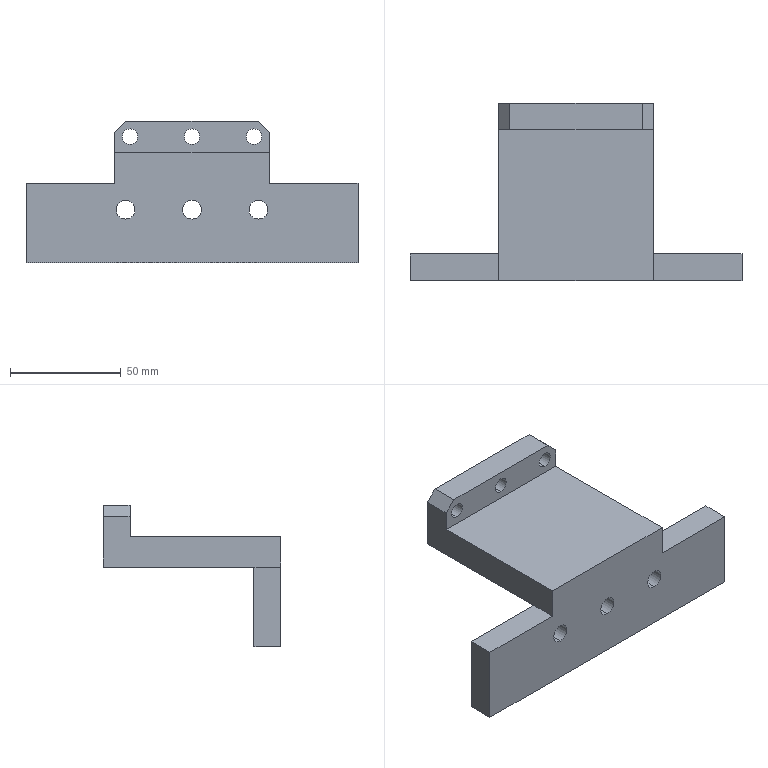NC program | NX | posted with a generic post | part box 150 x 80 x 64 mm
Whole program, first 2936 of 3152 lines:
N10 G17 G21 G94 G90
(FLOOR_WALL_COPY , TOOL : D63)
N12 T01 M6
N14 G54
N16 G17 G0 G90 X111.5 Y-41.997 B0. C0. S6500 M3
N18 G43 Z30. H1
N20 Z3.
N22 G94 G1 Z0. F1250.
N24 X108.5
N26 X-108.5
N28 Y-32.188
N30 Y-12.599
N32 X108.5
N34 Y16.8
N36 X-108.5
N38 X-111.5
N40 Z3.
N42 G0 Z30.
N44 M5
(FLOOR_WALL_2 , TOOL : D10)
N46 T10 M6
N48 G54
N50 G17 G0 G90 X1.443 Y-46.5 B0. C0. S9500 M3
N52 G43 Z30. H10
N54 Z1.001
N56 G94 G1 Z-0.499 F1000.
N58 X0.866 Y-45.5
N60 G3 X0. Y-45. R1.
N62 G1 X-40. F2500.
N64 Y22.9
N66 X40.
N68 Y-45.
N70 X0.
N72 Y-39.
N74 X-34.
N76 Y16.9
N78 X34.
N80 Y-39.
N82 X0.
N84 Y-33.
N86 X-28.
N88 Y10.9
N90 X28.
N92 Y-33.
N94 X0.
N96 Y-27.
N98 X-22.
N100 Y4.9
N102 X22.
N104 Y-27.
N106 X0.
N108 Y-21.
N110 X-16.
N112 Y-1.1
N114 X16.
N116 Y-21.
N118 X0.
N120 Y-15.
N122 X-10.
N124 Y-7.1
N126 X10.
N128 Y-15.
N130 X0.
N132 G3 X-0.866 Y-15.5 R1.
N134 G1 Z1.001
N136 G0 Z30.
N138 X1.443 Y-46.5
N140 Z0.503
N142 G1 Z-0.997 F1000.
N144 X0.866 Y-45.5
N146 G3 X0. Y-45. R1.
N148 G1 X-40. F2500.
N150 Y22.9
N152 X40.
N154 Y-45.
N156 X0.
N158 Y-39.
N160 X-34.
N162 Y16.9
N164 X34.
N166 Y-39.
N168 X0.
N170 Y-33.
N172 X-28.
N174 Y10.9
N176 X28.
N178 Y-33.
N180 X0.
N182 Y-27.
N184 X-22.
N186 Y4.9
N188 X22.
N190 Y-27.
N192 X0.
N194 Y-21.
N196 X-16.
N198 Y-1.1
N200 X16.
N202 Y-21.
N204 X0.
N206 Y-15.
N208 X-10.
N210 Y-7.1
N212 X10.
N214 Y-15.
N216 X0.
N218 G3 X-0.866 Y-15.5 R1.
N220 G1 Z0.503
N222 G0 Z30.
N224 X1.443 Y-46.5
N226 Z0.004
N228 G1 Z-1.496 F1000.
N230 X0.866 Y-45.5
N232 G3 X0. Y-45. R1.
N234 G1 X-40. F2500.
N236 Y22.9
N238 X40.
N240 Y-45.
N242 X0.
N244 Y-39.
N246 X-34.
N248 Y16.9
N250 X34.
N252 Y-39.
N254 X0.
N256 Y-33.
N258 X-28.
N260 Y10.9
N262 X28.
N264 Y-33.
N266 X0.
N268 Y-27.
N270 X-22.
N272 Y4.9
N274 X22.
N276 Y-27.
N278 X0.
N280 Y-21.
N282 X-16.
N284 Y-1.1
N286 X16.
N288 Y-21.
N290 X0.
N292 Y-15.
N294 X-10.
N296 Y-7.1
N298 X10.
N300 Y-15.
N302 X0.
N304 G3 X-0.866 Y-15.5 R1.
N306 G1 Z0.004
N308 G0 Z30.
N310 X1.443 Y-46.5
N312 Z-0.494
N314 G1 Z-1.994 F1000.
N316 X0.866 Y-45.5
N318 G3 X0. Y-45. R1.
N320 G1 X-40. F2500.
N322 Y22.9
N324 X40.
N326 Y-45.
N328 X0.
N330 Y-39.
N332 X-34.
N334 Y16.9
N336 X34.
N338 Y-39.
N340 X0.
N342 Y-33.
N344 X-28.
N346 Y10.9
N348 X28.
N350 Y-33.
N352 X0.
N354 Y-27.
N356 X-22.
N358 Y4.9
N360 X22.
N362 Y-27.
N364 X0.
N366 Y-21.
N368 X-16.
N370 Y-1.1
N372 X16.
N374 Y-21.
N376 X0.
N378 Y-15.
N380 X-10.
N382 Y-7.1
N384 X10.
N386 Y-15.
N388 X0.
N390 G3 X-0.866 Y-15.5 R1.
N392 G1 Z-0.494
N394 G0 Z30.
N396 X1.443 Y-46.5
N398 Z-0.993
N400 G1 Z-2.493 F1000.
N402 X0.866 Y-45.5
N404 G3 X0. Y-45. R1.
N406 G1 X-40. F2500.
N408 Y22.9
N410 X40.
N412 Y-45.
N414 X0.
N416 Y-39.
N418 X-34.
N420 Y16.9
N422 X34.
N424 Y-39.
N426 X0.
N428 Y-33.
N430 X-28.
N432 Y10.9
N434 X28.
N436 Y-33.
N438 X0.
N440 Y-27.
N442 X-22.
N444 Y4.9
N446 X22.
N448 Y-27.
N450 X0.
N452 Y-21.
N454 X-16.
N456 Y-1.1
N458 X16.
N460 Y-21.
N462 X0.
N464 Y-15.
N466 X-10.
N468 Y-7.1
N470 X10.
N472 Y-15.
N474 X0.
N476 G3 X-0.866 Y-15.5 R1.
N478 G1 Z-0.993
N480 G0 Z30.
N482 X1.443 Y-46.5
N484 Z-1.492
N486 G1 Z-2.992 F1000.
N488 X0.866 Y-45.5
N490 G3 X0. Y-45. R1.
N492 G1 X-40. F2500.
N494 Y22.9
N496 X40.
N498 Y-45.
N500 X0.
N502 Y-39.
N504 X-34.
N506 Y16.9
N508 X34.
N510 Y-39.
N512 X0.
N514 Y-33.
N516 X-28.
N518 Y10.9
N520 X28.
N522 Y-33.
N524 X0.
N526 Y-27.
N528 X-22.
N530 Y4.9
N532 X22.
N534 Y-27.
N536 X0.
N538 Y-21.
N540 X-16.
N542 Y-1.1
N544 X16.
N546 Y-21.
N548 X0.
N550 Y-15.
N552 X-10.
N554 Y-7.1
N556 X10.
N558 Y-15.
N560 X0.
N562 G3 X-0.866 Y-15.5 R1.
N564 G1 Z-1.492
N566 G0 Z30.
N568 X1.443 Y-46.5
N570 Z-1.99
N572 G1 Z-3.49 F1000.
N574 X0.866 Y-45.5
N576 G3 X0. Y-45. R1.
N578 G1 X-40. F2500.
N580 Y22.9
N582 X40.
N584 Y-45.
N586 X0.
N588 Y-39.
N590 X-34.
N592 Y16.9
N594 X34.
N596 Y-39.
N598 X0.
N600 Y-33.
N602 X-28.
N604 Y10.9
N606 X28.
N608 Y-33.
N610 X0.
N612 Y-27.
N614 X-22.
N616 Y4.9
N618 X22.
N620 Y-27.
N622 X0.
N624 Y-21.
N626 X-16.
N628 Y-1.1
N630 X16.
N632 Y-21.
N634 X0.
N636 Y-15.
N638 X-10.
N640 Y-7.1
N642 X10.
N644 Y-15.
N646 X0.
N648 G3 X-0.866 Y-15.5 R1.
N650 G1 Z-1.99
N652 G0 Z30.
N654 X1.443 Y-46.5
N656 Z-2.489
N658 G1 Z-3.989 F1000.
N660 X0.866 Y-45.5
N662 G3 X0. Y-45. R1.
N664 G1 X-40. F2500.
N666 Y22.9
N668 X40.
N670 Y-45.
N672 X0.
N674 Y-39.
N676 X-34.
N678 Y16.9
N680 X34.
N682 Y-39.
N684 X0.
N686 Y-33.
N688 X-28.
N690 Y10.9
N692 X28.
N694 Y-33.
N696 X0.
N698 Y-27.
N700 X-22.
N702 Y4.9
N704 X22.
N706 Y-27.
N708 X0.
N710 Y-21.
N712 X-16.
N714 Y-1.1
N716 X16.
N718 Y-21.
N720 X0.
N722 Y-15.
N724 X-10.
N726 Y-7.1
N728 X10.
N730 Y-15.
N732 X0.
N734 G3 X-0.866 Y-15.5 R1.
N736 G1 Z-2.489
N738 G0 Z30.
N740 X1.443 Y-46.5
N742 Z-2.988
N744 G1 Z-4.488 F1000.
N746 X0.866 Y-45.5
N748 G3 X0. Y-45. R1.
N750 G1 X-40. F2500.
N752 Y22.9
N754 X40.
N756 Y-45.
N758 X0.
N760 Y-39.
N762 X-34.
N764 Y16.9
N766 X34.
N768 Y-39.
N770 X0.
N772 Y-33.
N774 X-28.
N776 Y10.9
N778 X28.
N780 Y-33.
N782 X0.
N784 Y-27.
N786 X-22.
N788 Y4.9
N790 X22.
N792 Y-27.
N794 X0.
N796 Y-21.
N798 X-16.
N800 Y-1.1
N802 X16.
N804 Y-21.
N806 X0.
N808 Y-15.
N810 X-10.
N812 Y-7.1
N814 X10.
N816 Y-15.
N818 X0.
N820 G3 X-0.866 Y-15.5 R1.
N822 G1 Z-2.988
N824 G0 Z30.
N826 X1.443 Y-46.5
N828 Z-3.486
N830 G1 Z-4.986 F1000.
N832 X0.866 Y-45.5
N834 G3 X0. Y-45. R1.
N836 G1 X-40. F2500.
N838 Y22.9
N840 X40.
N842 Y-45.
N844 X0.
N846 Y-39.
N848 X-34.
N850 Y16.9
N852 X34.
N854 Y-39.
N856 X0.
N858 Y-33.
N860 X-28.
N862 Y10.9
N864 X28.
N866 Y-33.
N868 X0.
N870 Y-27.
N872 X-22.
N874 Y4.9
N876 X22.
N878 Y-27.
N880 X0.
N882 Y-21.
N884 X-16.
N886 Y-1.1
N888 X16.
N890 Y-21.
N892 X0.
N894 Y-15.
N896 X-10.
N898 Y-7.1
N900 X10.
N902 Y-15.
N904 X0.
N906 G3 X-0.866 Y-15.5 R1.
N908 G1 Z-3.486
N910 G0 Z30.
N912 X1.443 Y-46.5
N914 Z-3.985
N916 G1 Z-5.485 F1000.
N918 X0.866 Y-45.5
N920 G3 X0. Y-45. R1.
N922 G1 X-40. F2500.
N924 Y22.9
N926 X40.
N928 Y-45.
N930 X0.
N932 Y-39.
N934 X-34.
N936 Y16.9
N938 X34.
N940 Y-39.
N942 X0.
N944 Y-33.
N946 X-28.
N948 Y10.9
N950 X28.
N952 Y-33.
N954 X0.
N956 Y-27.
N958 X-22.
N960 Y4.9
N962 X22.
N964 Y-27.
N966 X0.
N968 Y-21.
N970 X-16.
N972 Y-1.1
N974 X16.
N976 Y-21.
N978 X0.
N980 Y-15.
N982 X-10.
N984 Y-7.1
N986 X10.
N988 Y-15.
N990 X0.
N992 G3 X-0.866 Y-15.5 R1.
N994 G1 Z-3.985
N996 G0 Z30.
N998 X1.443 Y-46.5
N1000 Z-4.483
N1002 G1 Z-5.983 F1000.
N1004 X0.866 Y-45.5
N1006 G3 X0. Y-45. R1.
N1008 G1 X-40. F2500.
N1010 Y22.9
N1012 X40.
N1014 Y-45.
N1016 X0.
N1018 Y-39.
N1020 X-34.
N1022 Y16.9
N1024 X34.
N1026 Y-39.
N1028 X0.
N1030 Y-33.
N1032 X-28.
N1034 Y10.9
N1036 X28.
N1038 Y-33.
N1040 X0.
N1042 Y-27.
N1044 X-22.
N1046 Y4.9
N1048 X22.
N1050 Y-27.
N1052 X0.
N1054 Y-21.
N1056 X-16.
N1058 Y-1.1
N1060 X16.
N1062 Y-21.
N1064 X0.
N1066 Y-15.
N1068 X-10.
N1070 Y-7.1
N1072 X10.
N1074 Y-15.
N1076 X0.
N1078 G3 X-0.866 Y-15.5 R1.
N1080 G1 Z-4.483
N1082 G0 Z30.
N1084 X1.443 Y-46.5
N1086 Z-4.982
N1088 G1 Z-6.482 F1000.
N1090 X0.866 Y-45.5
N1092 G3 X0. Y-45. R1.
N1094 G1 X-40. F2500.
N1096 Y22.9
N1098 X40.
N1100 Y-45.
N1102 X0.
N1104 Y-39.
N1106 X-34.
N1108 Y16.9
N1110 X34.
N1112 Y-39.
N1114 X0.
N1116 Y-33.
N1118 X-28.
N1120 Y10.9
N1122 X28.
N1124 Y-33.
N1126 X0.
N1128 Y-27.
N1130 X-22.
N1132 Y4.9
N1134 X22.
N1136 Y-27.
N1138 X0.
N1140 Y-21.
N1142 X-16.
N1144 Y-1.1
N1146 X16.
N1148 Y-21.
N1150 X0.
N1152 Y-15.
N1154 X-10.
N1156 Y-7.1
N1158 X10.
N1160 Y-15.
N1162 X0.
N1164 G3 X-0.866 Y-15.5 R1.
N1166 G1 Z-4.982
N1168 G0 Z30.
N1170 X1.443 Y-46.5
N1172 Z-5.481
N1174 G1 Z-6.981 F1000.
N1176 X0.866 Y-45.5
N1178 G3 X0. Y-45. R1.
N1180 G1 X-40. F2500.
N1182 Y22.9
N1184 X40.
N1186 Y-45.
N1188 X0.
N1190 Y-39.
N1192 X-34.
N1194 Y16.9
N1196 X34.
N1198 Y-39.
N1200 X0.
N1202 Y-33.
N1204 X-28.
N1206 Y10.9
N1208 X28.
N1210 Y-33.
N1212 X0.
N1214 Y-27.
N1216 X-22.
N1218 Y4.9
N1220 X22.
N1222 Y-27.
N1224 X0.
N1226 Y-21.
N1228 X-16.
N1230 Y-1.1
N1232 X16.
N1234 Y-21.
N1236 X0.
N1238 Y-15.
N1240 X-10.
N1242 Y-7.1
N1244 X10.
N1246 Y-15.
N1248 X0.
N1250 G3 X-0.866 Y-15.5 R1.
N1252 G1 Z-5.481
N1254 G0 Z30.
N1256 X1.443 Y-46.5
N1258 Z-5.979
N1260 G1 Z-7.479 F1000.
N1262 X0.866 Y-45.5
N1264 G3 X0. Y-45. R1.
N1266 G1 X-40. F2500.
N1268 Y22.9
N1270 X40.
N1272 Y-45.
N1274 X0.
N1276 Y-39.
N1278 X-34.
N1280 Y16.9
N1282 X34.
N1284 Y-39.
N1286 X0.
N1288 Y-33.
N1290 X-28.
N1292 Y10.9
N1294 X28.
N1296 Y-33.
N1298 X0.
N1300 Y-27.
N1302 X-22.
N1304 Y4.9
N1306 X22.
N1308 Y-27.
N1310 X0.
N1312 Y-21.
N1314 X-16.
N1316 Y-1.1
N1318 X16.
N1320 Y-21.
N1322 X0.
N1324 Y-15.
N1326 X-10.
N1328 Y-7.1
N1330 X10.
N1332 Y-15.
N1334 X0.
N1336 G3 X-0.866 Y-15.5 R1.
N1338 G1 Z-5.979
N1340 G0 Z30.
N1342 X1.443 Y-46.5
N1344 Z-6.478
N1346 G1 Z-7.978 F1000.
N1348 X0.866 Y-45.5
N1350 G3 X0. Y-45. R1.
N1352 G1 X-40. F2500.
N1354 Y22.9
N1356 X40.
N1358 Y-45.
N1360 X0.
N1362 Y-39.
N1364 X-34.
N1366 Y16.9
N1368 X34.
N1370 Y-39.
N1372 X0.
N1374 Y-33.
N1376 X-28.
N1378 Y10.9
N1380 X28.
N1382 Y-33.
N1384 X0.
N1386 Y-27.
N1388 X-22.
N1390 Y4.9
N1392 X22.
N1394 Y-27.
N1396 X0.
N1398 Y-21.
N1400 X-16.
N1402 Y-1.1
N1404 X16.
N1406 Y-21.
N1408 X0.
N1410 Y-15.
N1412 X-10.
N1414 Y-7.1
N1416 X10.
N1418 Y-15.
N1420 X0.
N1422 G3 X-0.866 Y-15.5 R1.
N1424 G1 Z-6.478
N1426 G0 Z30.
N1428 X1.443 Y-46.5
N1430 Z-6.976
N1432 G1 Z-8.476 F1000.
N1434 X0.866 Y-45.5
N1436 G3 X0. Y-45. R1.
N1438 G1 X-40. F2500.
N1440 Y22.9
N1442 X40.
N1444 Y-45.
N1446 X0.
N1448 Y-39.
N1450 X-34.
N1452 Y16.9
N1454 X34.
N1456 Y-39.
N1458 X0.
N1460 Y-33.
N1462 X-28.
N1464 Y10.9
N1466 X28.
N1468 Y-33.
N1470 X0.
N1472 Y-27.
N1474 X-22.
N1476 Y4.9
N1478 X22.
N1480 Y-27.
N1482 X0.
N1484 Y-21.
N1486 X-16.
N1488 Y-1.1
N1490 X16.
N1492 Y-21.
N1494 X0.
N1496 Y-15.
N1498 X-10.
N1500 Y-7.1
N1502 X10.
N1504 Y-15.
N1506 X0.
N1508 G3 X-0.866 Y-15.5 R1.
N1510 G1 Z-6.976
N1512 G0 Z30.
N1514 X1.443 Y-46.5
N1516 Z-7.475
N1518 G1 Z-8.975 F1000.
N1520 X0.866 Y-45.5
N1522 G3 X0. Y-45. R1.
N1524 G1 X-40. F2500.
N1526 Y22.9
N1528 X40.
N1530 Y-45.
N1532 X0.
N1534 Y-39.
N1536 X-34.
N1538 Y16.9
N1540 X34.
N1542 Y-39.
N1544 X0.
N1546 Y-33.
N1548 X-28.
N1550 Y10.9
N1552 X28.
N1554 Y-33.
N1556 X0.
N1558 Y-27.
N1560 X-22.
N1562 Y4.9
N1564 X22.
N1566 Y-27.
N1568 X0.
N1570 Y-21.
N1572 X-16.
N1574 Y-1.1
N1576 X16.
N1578 Y-21.
N1580 X0.
N1582 Y-15.
N1584 X-10.
N1586 Y-7.1
N1588 X10.
N1590 Y-15.
N1592 X0.
N1594 G3 X-0.866 Y-15.5 R1.
N1596 G1 Z-7.475
N1598 G0 Z30.
N1600 X1.443 Y-46.5
N1602 Z-7.974
N1604 G1 Z-9.474 F1000.
N1606 X0.866 Y-45.5
N1608 G3 X0. Y-45. R1.
N1610 G1 X-40. F2500.
N1612 Y22.9
N1614 X40.
N1616 Y-45.
N1618 X0.
N1620 Y-39.
N1622 X-34.
N1624 Y16.9
N1626 X34.
N1628 Y-39.
N1630 X0.
N1632 Y-33.
N1634 X-28.
N1636 Y10.9
N1638 X28.
N1640 Y-33.
N1642 X0.
N1644 Y-27.
N1646 X-22.
N1648 Y4.9
N1650 X22.
N1652 Y-27.
N1654 X0.
N1656 Y-21.
N1658 X-16.
N1660 Y-1.1
N1662 X16.
N1664 Y-21.
N1666 X0.
N1668 Y-15.
N1670 X-10.
N1672 Y-7.1
N1674 X10.
N1676 Y-15.
N1678 X0.
N1680 G3 X-0.866 Y-15.5 R1.
N1682 G1 Z-7.974
N1684 G0 Z30.
N1686 X1.443 Y-46.5
N1688 Z-8.472
N1690 G1 Z-9.972 F1000.
N1692 X0.866 Y-45.5
N1694 G3 X0. Y-45. R1.
N1696 G1 X-40. F2500.
N1698 Y22.9
N1700 X40.
N1702 Y-45.
N1704 X0.
N1706 Y-39.
N1708 X-34.
N1710 Y16.9
N1712 X34.
N1714 Y-39.
N1716 X0.
N1718 Y-33.
N1720 X-28.
N1722 Y10.9
N1724 X28.
N1726 Y-33.
N1728 X0.
N1730 Y-27.
N1732 X-22.
N1734 Y4.9
N1736 X22.
N1738 Y-27.
N1740 X0.
N1742 Y-21.
N1744 X-16.
N1746 Y-1.1
N1748 X16.
N1750 Y-21.
N1752 X0.
N1754 Y-15.
N1756 X-10.
N1758 Y-7.1
N1760 X10.
N1762 Y-15.
N1764 X0.
N1766 G3 X-0.866 Y-15.5 R1.
N1768 G1 Z-8.472
N1770 G0 Z30.
N1772 X1.443 Y-46.5
N1774 Z-8.971
N1776 G1 Z-10.471 F1000.
N1778 X0.866 Y-45.5
N1780 G3 X0. Y-45. R1.
N1782 G1 X-40. F2500.
N1784 Y22.9
N1786 X40.
N1788 Y-45.
N1790 X0.
N1792 Y-39.
N1794 X-34.
N1796 Y16.9
N1798 X34.
N1800 Y-39.
N1802 X0.
N1804 Y-33.
N1806 X-28.
N1808 Y10.9
N1810 X28.
N1812 Y-33.
N1814 X0.
N1816 Y-27.
N1818 X-22.
N1820 Y4.9
N1822 X22.
N1824 Y-27.
N1826 X0.
N1828 Y-21.
N1830 X-16.
N1832 Y-1.1
N1834 X16.
N1836 Y-21.
N1838 X0.
N1840 Y-15.
N1842 X-10.
N1844 Y-7.1
N1846 X10.
N1848 Y-15.
N1850 X0.
N1852 G3 X-0.866 Y-15.5 R1.
N1854 G1 Z-8.971
N1856 G0 Z30.
N1858 X1.443 Y-46.5
N1860 Z-9.469
N1862 G1 Z-10.969 F1000.
N1864 X0.866 Y-45.5
N1866 G3 X0. Y-45. R1.
N1868 G1 X-40. F2500.
N1870 Y22.9
N1872 X40.
N1874 Y-45.
N1876 X0.
N1878 Y-39.
N1880 X-34.
N1882 Y16.9
N1884 X34.
N1886 Y-39.
N1888 X0.
N1890 Y-33.
N1892 X-28.
N1894 Y10.9
N1896 X28.
N1898 Y-33.
N1900 X0.
N1902 Y-27.
N1904 X-22.
N1906 Y4.9
N1908 X22.
N1910 Y-27.
N1912 X0.
N1914 Y-21.
N1916 X-16.
N1918 Y-1.1
N1920 X16.
N1922 Y-21.
N1924 X0.
N1926 Y-15.
N1928 X-10.
N1930 Y-7.1
N1932 X10.
N1934 Y-15.
N1936 X0.
N1938 G3 X-0.866 Y-15.5 R1.
N1940 G1 Z-9.469
N1942 G0 Z30.
N1944 X1.443 Y-46.5
N1946 Z-9.968
N1948 G1 Z-11.468 F1000.
N1950 X0.866 Y-45.5
N1952 G3 X0. Y-45. R1.
N1954 G1 X-40. F2500.
N1956 Y22.9
N1958 X40.
N1960 Y-45.
N1962 X0.
N1964 Y-39.
N1966 X-34.
N1968 Y16.9
N1970 X34.
N1972 Y-39.
N1974 X0.
N1976 Y-33.
N1978 X-28.
N1980 Y10.9
N1982 X28.
N1984 Y-33.
N1986 X0.
N1988 Y-27.
N1990 X-22.
N1992 Y4.9
N1994 X22.
N1996 Y-27.
N1998 X0.
N2000 Y-21.
N2002 X-16.
N2004 Y-1.1
N2006 X16.
N2008 Y-21.
N2010 X0.
N2012 Y-15.
N2014 X-10.
N2016 Y-7.1
N2018 X10.
N2020 Y-15.
N2022 X0.
N2024 G3 X-0.866 Y-15.5 R1.
N2026 G1 Z-9.968
N2028 G0 Z30.
N2030 X1.443 Y-46.5
N2032 Z-10.467
N2034 G1 Z-11.967 F1000.
N2036 X0.866 Y-45.5
N2038 G3 X0. Y-45. R1.
N2040 G1 X-40. F2500.
N2042 Y22.9
N2044 X40.
N2046 Y-45.
N2048 X0.
N2050 Y-39.
N2052 X-34.
N2054 Y16.9
N2056 X34.
N2058 Y-39.
N2060 X0.
N2062 Y-33.
N2064 X-28.
N2066 Y10.9
N2068 X28.
N2070 Y-33.
N2072 X0.
N2074 Y-27.
N2076 X-22.
N2078 Y4.9
N2080 X22.
N2082 Y-27.
N2084 X0.
N2086 Y-21.
N2088 X-16.
N2090 Y-1.1
N2092 X16.
N2094 Y-21.
N2096 X0.
N2098 Y-15.
N2100 X-10.
N2102 Y-7.1
N2104 X10.
N2106 Y-15.
N2108 X0.
N2110 G3 X-0.866 Y-15.5 R1.
N2112 G1 Z-10.467
N2114 G0 Z30.
N2116 X1.443 Y-46.5
N2118 Z-10.965
N2120 G1 Z-12.465 F1000.
N2122 X0.866 Y-45.5
N2124 G3 X0. Y-45. R1.
N2126 G1 X-40. F2500.
N2128 Y22.9
N2130 X40.
N2132 Y-45.
N2134 X0.
N2136 Y-39.
N2138 X-34.
N2140 Y16.9
N2142 X34.
N2144 Y-39.
N2146 X0.
N2148 Y-33.
N2150 X-28.
N2152 Y10.9
N2154 X28.
N2156 Y-33.
N2158 X0.
N2160 Y-27.
N2162 X-22.
N2164 Y4.9
N2166 X22.
N2168 Y-27.
N2170 X0.
N2172 Y-21.
N2174 X-16.
N2176 Y-1.1
N2178 X16.
N2180 Y-21.
N2182 X0.
N2184 Y-15.
N2186 X-10.
N2188 Y-7.1
N2190 X10.
N2192 Y-15.
N2194 X0.
N2196 G3 X-0.866 Y-15.5 R1.
N2198 G1 Z-10.965
N2200 G0 Z30.
N2202 X1.443 Y-46.5
N2204 Z-11.464
N2206 G1 Z-12.964 F1000.
N2208 X0.866 Y-45.5
N2210 G3 X0. Y-45. R1.
N2212 G1 X-40. F2500.
N2214 Y22.9
N2216 X40.
N2218 Y-45.
N2220 X0.
N2222 Y-39.
N2224 X-34.
N2226 Y16.9
N2228 X34.
N2230 Y-39.
N2232 X0.
N2234 Y-33.
N2236 X-28.
N2238 Y10.9
N2240 X28.
N2242 Y-33.
N2244 X0.
N2246 Y-27.
N2248 X-22.
N2250 Y4.9
N2252 X22.
N2254 Y-27.
N2256 X0.
N2258 Y-21.
N2260 X-16.
N2262 Y-1.1
N2264 X16.
N2266 Y-21.
N2268 X0.
N2270 Y-15.
N2272 X-10.
N2274 Y-7.1
N2276 X10.
N2278 Y-15.
N2280 X0.
N2282 G3 X-0.866 Y-15.5 R1.
N2284 G1 Z-11.464
N2286 G0 Z30.
N2288 X1.443 Y-46.5
N2290 Z-11.963
N2292 G1 Z-13.463 F1000.
N2294 X0.866 Y-45.5
N2296 G3 X0. Y-45. R1.
N2298 G1 X-40. F2500.
N2300 Y22.9
N2302 X40.
N2304 Y-45.
N2306 X0.
N2308 Y-39.
N2310 X-34.
N2312 Y16.9
N2314 X34.
N2316 Y-39.
N2318 X0.
N2320 Y-33.
N2322 X-28.
N2324 Y10.9
N2326 X28.
N2328 Y-33.
N2330 X0.
N2332 Y-27.
N2334 X-22.
N2336 Y4.9
N2338 X22.
N2340 Y-27.
N2342 X0.
N2344 Y-21.
N2346 X-16.
N2348 Y-1.1
N2350 X16.
N2352 Y-21.
N2354 X0.
N2356 Y-15.
N2358 X-10.
N2360 Y-7.1
N2362 X10.
N2364 Y-15.
N2366 X0.
N2368 G3 X-0.866 Y-15.5 R1.
N2370 G1 Z-11.963
N2372 G0 Z30.
N2374 X1.443 Y-46.5
N2376 Z-12.461
N2378 G1 Z-13.961 F1000.
N2380 X0.866 Y-45.5
N2382 G3 X0. Y-45. R1.
N2384 G1 X-40. F2500.
N2386 Y22.9
N2388 X40.
N2390 Y-45.
N2392 X0.
N2394 Y-39.
N2396 X-34.
N2398 Y16.9
N2400 X34.
N2402 Y-39.
N2404 X0.
N2406 Y-33.
N2408 X-28.
N2410 Y10.9
N2412 X28.
N2414 Y-33.
N2416 X0.
N2418 Y-27.
N2420 X-22.
N2422 Y4.9
N2424 X22.
N2426 Y-27.
N2428 X0.
N2430 Y-21.
N2432 X-16.
N2434 Y-1.1
N2436 X16.
N2438 Y-21.
N2440 X0.
N2442 Y-15.
N2444 X-10.
N2446 Y-7.1
N2448 X10.
N2450 Y-15.
N2452 X0.
N2454 G3 X-0.866 Y-15.5 R1.
N2456 G1 Z-12.461
N2458 G0 Z30.
N2460 X1.443 Y-46.5
N2462 Z-12.96
N2464 G1 Z-14.46 F1000.
N2466 X0.866 Y-45.5
N2468 G3 X0. Y-45. R1.
N2470 G1 X-40. F2500.
N2472 Y22.9
N2474 X40.
N2476 Y-45.
N2478 X0.
N2480 Y-39.
N2482 X-34.
N2484 Y16.9
N2486 X34.
N2488 Y-39.
N2490 X0.
N2492 Y-33.
N2494 X-28.
N2496 Y10.9
N2498 X28.
N2500 Y-33.
N2502 X0.
N2504 Y-27.
N2506 X-22.
N2508 Y4.9
N2510 X22.
N2512 Y-27.
N2514 X0.
N2516 Y-21.
N2518 X-16.
N2520 Y-1.1
N2522 X16.
N2524 Y-21.
N2526 X0.
N2528 Y-15.
N2530 X-10.
N2532 Y-7.1
N2534 X10.
N2536 Y-15.
N2538 X0.
N2540 G3 X-0.866 Y-15.5 R1.
N2542 G1 Z-12.96
N2544 G0 Z30.
N2546 X1.443 Y-46.5
N2548 Z-13.458
N2550 G1 Z-14.958 F1000.
N2552 X0.866 Y-45.5
N2554 G3 X0. Y-45. R1.
N2556 G1 X-40. F2500.
N2558 Y22.9
N2560 X40.
N2562 Y-45.
N2564 X0.
N2566 Y-39.
N2568 X-34.
N2570 Y16.9
N2572 X34.
N2574 Y-39.
N2576 X0.
N2578 Y-33.
N2580 X-28.
N2582 Y10.9
N2584 X28.
N2586 Y-33.
N2588 X0.
N2590 Y-27.
N2592 X-22.
N2594 Y4.9
N2596 X22.
N2598 Y-27.
N2600 X0.
N2602 Y-21.
N2604 X-16.
N2606 Y-1.1
N2608 X16.
N2610 Y-21.
N2612 X0.
N2614 Y-15.
N2616 X-10.
N2618 Y-7.1
N2620 X10.
N2622 Y-15.
N2624 X0.
N2626 G3 X-0.866 Y-15.5 R1.
N2628 G1 Z-13.458
N2630 G0 Z30.
N2632 X1.443 Y-46.5
N2634 Z-13.957
N2636 G1 Z-15.457 F1000.
N2638 X0.866 Y-45.5
N2640 G3 X0. Y-45. R1.
N2642 G1 X-40. F2500.
N2644 Y22.9
N2646 X40.
N2648 Y-45.
N2650 X0.
N2652 Y-39.
N2654 X-34.
N2656 Y16.9
N2658 X34.
N2660 Y-39.
N2662 X0.
N2664 Y-33.
N2666 X-28.
N2668 Y10.9
N2670 X28.
N2672 Y-33.
N2674 X0.
N2676 Y-27.
N2678 X-22.
N2680 Y4.9
N2682 X22.
N2684 Y-27.
N2686 X0.
N2688 Y-21.
N2690 X-16.
N2692 Y-1.1
N2694 X16.
N2696 Y-21.
N2698 X0.
N2700 Y-15.
N2702 X-10.
N2704 Y-7.1
N2706 X10.
N2708 Y-15.
N2710 X0.
N2712 G3 X-0.866 Y-15.5 R1.
N2714 G1 Z-13.957
N2716 G0 Z30.
N2718 X1.443 Y-46.5
N2720 Z-14.456
N2722 G1 Z-15.956 F1000.
N2724 X0.866 Y-45.5
N2726 G3 X0. Y-45. R1.
N2728 G1 X-40. F2500.
N2730 Y22.9
N2732 X40.
N2734 Y-45.
N2736 X0.
N2738 Y-39.
N2740 X-34.
N2742 Y16.9
N2744 X34.
N2746 Y-39.
N2748 X0.
N2750 Y-33.
N2752 X-28.
N2754 Y10.9
N2756 X28.
N2758 Y-33.
N2760 X0.
N2762 Y-27.
N2764 X-22.
N2766 Y4.9
N2768 X22.
N2770 Y-27.
N2772 X0.
N2774 Y-21.
N2776 X-16.
N2778 Y-1.1
N2780 X16.
N2782 Y-21.
N2784 X0.
N2786 Y-15.
N2788 X-10.
N2790 Y-7.1
N2792 X10.
N2794 Y-15.
N2796 X0.
N2798 G3 X-0.866 Y-15.5 R1.
N2800 G1 Z-14.456
N2802 G0 Z30.
N2804 X1.443 Y-46.5
N2806 Z-14.954
N2808 G1 Z-16.454 F1000.
N2810 X0.866 Y-45.5
N2812 G3 X0. Y-45. R1.
N2814 G1 X-40. F2500.
N2816 Y22.9
N2818 X40.
N2820 Y-45.
N2822 X0.
N2824 Y-39.
N2826 X-34.
N2828 Y16.9
N2830 X34.
N2832 Y-39.
N2834 X0.
N2836 Y-33.
N2838 X-28.
N2840 Y10.9
N2842 X28.
N2844 Y-33.
N2846 X0.
N2848 Y-27.
N2850 X-22.
N2852 Y4.9
N2854 X22.
N2856 Y-27.
N2858 X0.
N2860 Y-21.
N2862 X-16.
N2864 Y-1.1
N2866 X16.
N2868 Y-21.
N2870 X0.
N2872 Y-15.
N2874 X-10.
N2876 Y-7.1
N2878 X10.
N2880 Y-15.
N2882 X0.
N2884 G3 X-0.866 Y-15.5 R1.
N2886 G1 Z-14.954
N2888 G0 Z30.
N2890 X1.443 Y-46.5
N2892 Z-15.453
N2894 G1 Z-16.953 F1000.
N2896 X0.866 Y-45.5
N2898 G3 X0. Y-45. R1.
N2900 G1 X-40. F2500.
N2902 Y22.9
N2904 X40.
N2906 Y-45.
N2908 X0.
N2910 Y-39.
N2912 X-34.
N2914 Y16.9
N2916 X34.
N2918 Y-39.
N2920 X0.
N2922 Y-33.
N2924 X-28.
N2926 Y10.9
N2928 X28.
N2930 Y-33.
N2932 X0.
N2934 Y-27.
N2936 X-22.
N2938 Y4.9
N2940 X22.
N2942 Y-27.
N2944 X0.
N2946 Y-21.
N2948 X-16.
N2950 Y-1.1
N2952 X16.
N2954 Y-21.
N2956 X0.
N2958 Y-15.
N2960 X-10.
N2962 Y-7.1
N2964 X10.
N2966 Y-15.
N2968 X0.
N2970 G3 X-0.866 Y-15.5 R1.
N2972 G1 Z-15.453
N2974 G0 Z30.
N2976 X1.443 Y-46.5
N2978 Z-15.951
N2980 G1 Z-17.451 F1000.
N2982 X0.866 Y-45.5
N2984 G3 X0. Y-45. R1.
N2986 G1 X-40. F2500.
N2988 Y22.9
N2990 X40.
N2992 Y-45.
N2994 X0.
N2996 Y-39.
N2998 X-34.
N3000 Y16.9
N3002 X34.
N3004 Y-39.
N3006 X0.
N3008 Y-33.
N3010 X-28.
N3012 Y10.9
N3014 X28.
N3016 Y-33.
N3018 X0.
N3020 Y-27.
N3022 X-22.
N3024 Y4.9
N3026 X22.
N3028 Y-27.
N3030 X0.
N3032 Y-21.
N3034 X-16.
N3036 Y-1.1
N3038 X16.
N3040 Y-21.
N3042 X0.
N3044 Y-15.
N3046 X-10.
N3048 Y-7.1
N3050 X10.
N3052 Y-15.
N3054 X0.
N3056 G3 X-0.866 Y-15.5 R1.
N3058 G1 Z-15.951
N3060 G0 Z30.
N3062 X1.443 Y-46.5
N3064 Z-16.45
N3066 G1 Z-17.95 F1000.
N3068 X0.866 Y-45.5
N3070 G3 X0. Y-45. R1.
N3072 G1 X-40. F2500.
N3074 Y22.9
N3076 X40.
N3078 Y-45.
N3080 X0.
N3082 Y-39.
N3084 X-34.
N3086 Y16.9
N3088 X34.
N3090 Y-39.
N3092 X0.
N3094 Y-33.
N3096 X-28.
N3098 Y10.9
N3100 X28.
N3102 Y-33.
N3104 X0.
N3106 Y-27.
N3108 X-22.
N3110 Y4.9
N3112 X22.
N3114 Y-27.
N3116 X0.
N3118 Y-21.
N3120 X-16.
N3122 Y-1.1
N3124 X16.
N3126 Y-21.
N3128 X0.
N3130 Y-15.
N3132 X-10.
N3134 Y-7.1
N3136 X10.
N3138 Y-15.
N3140 X0.
N3142 G3 X-0.866 Y-15.5 R1.
N3144 G1 Z-16.45
N3146 G0 Z30.
N3148 X1.443 Y-46.5
N3150 Z-16.949
N3152 G1 Z-18.449 F1000.
N3154 X0.866 Y-45.5
N3156 G3 X0. Y-45. R1.
N3158 G1 X-40. F2500.
N3160 Y22.9
N3162 X40.
N3164 Y-45.
N3166 X0.
N3168 Y-39.
N3170 X-34.
N3172 Y16.9
N3174 X34.
N3176 Y-39.
N3178 X0.
N3180 Y-33.
N3182 X-28.
N3184 Y10.9
N3186 X28.
N3188 Y-33.
N3190 X0.
N3192 Y-27.
N3194 X-22.
N3196 Y4.9
N3198 X22.
N3200 Y-27.
N3202 X0.
N3204 Y-21.
N3206 X-16.
N3208 Y-1.1
N3210 X16.
N3212 Y-21.
N3214 X0.
N3216 Y-15.
N3218 X-10.
N3220 Y-7.1
N3222 X10.
N3224 Y-15.
N3226 X0.
N3228 G3 X-0.866 Y-15.5 R1.
N3230 G1 Z-16.949
N3232 G0 Z30.
N3234 X1.443 Y-46.5
N3236 Z-17.447
N3238 G1 Z-18.947 F1000.
N3240 X0.866 Y-45.5
N3242 G3 X0. Y-45. R1.
N3244 G1 X-40. F2500.
N3246 Y22.9
N3248 X40.
N3250 Y-45.
N3252 X0.
N3254 Y-39.
N3256 X-34.
N3258 Y16.9
N3260 X34.
N3262 Y-39.
N3264 X0.
N3266 Y-33.
N3268 X-28.
N3270 Y10.9
N3272 X28.
N3274 Y-33.
N3276 X0.
N3278 Y-27.
N3280 X-22.
N3282 Y4.9
N3284 X22.
N3286 Y-27.
N3288 X0.
N3290 Y-21.
N3292 X-16.
N3294 Y-1.1
N3296 X16.
N3298 Y-21.
N3300 X0.
N3302 Y-15.
N3304 X-10.
N3306 Y-7.1
N3308 X10.
N3310 Y-15.
N3312 X0.
N3314 G3 X-0.866 Y-15.5 R1.
N3316 G1 Z-17.447
N3318 G0 Z30.
N3320 X1.443 Y-46.5
N3322 Z-17.946
N3324 G1 Z-19.446 F1000.
N3326 X0.866 Y-45.5
N3328 G3 X0. Y-45. R1.
N3330 G1 X-40. F2500.
N3332 Y22.9
N3334 X40.
N3336 Y-45.
N3338 X0.
N3340 Y-39.
N3342 X-34.
N3344 Y16.9
N3346 X34.
N3348 Y-39.
N3350 X0.
N3352 Y-33.
N3354 X-28.
N3356 Y10.9
N3358 X28.
N3360 Y-33.
N3362 X0.
N3364 Y-27.
N3366 X-22.
N3368 Y4.9
N3370 X22.
N3372 Y-27.
N3374 X0.
N3376 Y-21.
N3378 X-16.
N3380 Y-1.1
N3382 X16.
N3384 Y-21.
N3386 X0.
N3388 Y-15.
N3390 X-10.
N3392 Y-7.1
N3394 X10.
N3396 Y-15.
N3398 X0.
N3400 G3 X-0.866 Y-15.5 R1.
N3402 G1 Z-17.946
N3404 G0 Z30.
N3406 X1.443 Y-46.5
N3408 Z-18.444
N3410 G1 Z-19.944 F1000.
N3412 X0.866 Y-45.5
N3414 G3 X0. Y-45. R1.
N3416 G1 X-40. F2500.
N3418 Y22.9
N3420 X40.
N3422 Y-45.
N3424 X0.
N3426 Y-39.
N3428 X-34.
N3430 Y16.9
N3432 X34.
N3434 Y-39.
N3436 X0.
N3438 Y-33.
N3440 X-28.
N3442 Y10.9
N3444 X28.
N3446 Y-33.
N3448 X0.
N3450 Y-27.
N3452 X-22.
N3454 Y4.9
N3456 X22.
N3458 Y-27.
N3460 X0.
N3462 Y-21.
N3464 X-16.
N3466 Y-1.1
N3468 X16.
N3470 Y-21.
N3472 X0.
N3474 Y-15.
N3476 X-10.
N3478 Y-7.1
N3480 X10.
N3482 Y-15.
N3484 X0.
N3486 G3 X-0.866 Y-15.5 R1.
N3488 G1 Z-18.444
N3490 G0 Z30.
N3492 X1.443 Y-46.5
N3494 Z-18.943
N3496 G1 Z-20.443 F1000.
N3498 X0.866 Y-45.5
N3500 G3 X0. Y-45. R1.
N3502 G1 X-40. F2500.
N3504 Y22.9
N3506 X40.
N3508 Y-45.
N3510 X0.
N3512 Y-39.
N3514 X-34.
N3516 Y16.9
N3518 X34.
N3520 Y-39.
N3522 X0.
N3524 Y-33.
N3526 X-28.
N3528 Y10.9
N3530 X28.
N3532 Y-33.
N3534 X0.
N3536 Y-27.
N3538 X-22.
N3540 Y4.9
N3542 X22.
N3544 Y-27.
N3546 X0.
N3548 Y-21.
N3550 X-16.
N3552 Y-1.1
N3554 X16.
N3556 Y-21.
N3558 X0.
N3560 Y-15.
N3562 X-10.
N3564 Y-7.1
N3566 X10.
N3568 Y-15.
N3570 X0.
N3572 G3 X-0.866 Y-15.5 R1.
N3574 G1 Z-18.943
N3576 G0 Z30.
N3578 X1.443 Y-46.5
N3580 Z-19.442
N3582 G1 Z-20.942 F1000.
N3584 X0.866 Y-45.5
N3586 G3 X0. Y-45. R1.
N3588 G1 X-40. F2500.
N3590 Y22.9
N3592 X40.
N3594 Y-45.
N3596 X0.
N3598 Y-39.
N3600 X-34.
N3602 Y16.9
N3604 X34.
N3606 Y-39.
N3608 X0.
N3610 Y-33.
N3612 X-28.
N3614 Y10.9
N3616 X28.
N3618 Y-33.
N3620 X0.
N3622 Y-27.
N3624 X-22.
N3626 Y4.9
N3628 X22.
N3630 Y-27.
N3632 X0.
N3634 Y-21.
N3636 X-16.
N3638 Y-1.1
N3640 X16.
N3642 Y-21.
N3644 X0.
N3646 Y-15.
N3648 X-10.
N3650 Y-7.1
N3652 X10.
N3654 Y-15.
N3656 X0.
N3658 G3 X-0.866 Y-15.5 R1.
N3660 G1 Z-19.442
N3662 G0 Z30.
N3664 X1.443 Y-46.5
N3666 Z-19.94
N3668 G1 Z-21.44 F1000.
N3670 X0.866 Y-45.5
N3672 G3 X0. Y-45. R1.
N3674 G1 X-40. F2500.
N3676 Y22.9
N3678 X40.
N3680 Y-45.
N3682 X0.
N3684 Y-39.
N3686 X-34.
N3688 Y16.9
N3690 X34.
N3692 Y-39.
N3694 X0.
N3696 Y-33.
N3698 X-28.
N3700 Y10.9
N3702 X28.
N3704 Y-33.
N3706 X0.
N3708 Y-27.
N3710 X-22.
N3712 Y4.9
N3714 X22.
N3716 Y-27.
N3718 X0.
N3720 Y-21.
N3722 X-16.
N3724 Y-1.1
N3726 X16.
N3728 Y-21.
N3730 X0.
N3732 Y-15.
N3734 X-10.
N3736 Y-7.1
N3738 X10.
N3740 Y-15.
N3742 X0.
N3744 G3 X-0.866 Y-15.5 R1.
N3746 G1 Z-19.94
N3748 G0 Z30.
N3750 X1.443 Y-46.5
N3752 Z-20.439
N3754 G1 Z-21.939 F1000.
N3756 X0.866 Y-45.5
N3758 G3 X0. Y-45. R1.
N3760 G1 X-40. F2500.
N3762 Y22.9
N3764 X40.
N3766 Y-45.
N3768 X0.
N3770 Y-39.
N3772 X-34.
N3774 Y16.9
N3776 X34.
N3778 Y-39.
N3780 X0.
N3782 Y-33.
N3784 X-28.
N3786 Y10.9
N3788 X28.
N3790 Y-33.
N3792 X0.
N3794 Y-27.
N3796 X-22.
N3798 Y4.9
N3800 X22.
N3802 Y-27.
N3804 X0.
N3806 Y-21.
N3808 X-16.
N3810 Y-1.1
N3812 X16.
N3814 Y-21.
N3816 X0.
N3818 Y-15.
N3820 X-10.
N3822 Y-7.1
N3824 X10.
N3826 Y-15.
N3828 X0.
N3830 G3 X-0.866 Y-15.5 R1.
N3832 G1 Z-20.439
N3834 G0 Z30.
N3836 X1.443 Y-46.5
N3838 Z-20.938
N3840 G1 Z-22.438 F1000.
N3842 X0.866 Y-45.5
N3844 G3 X0. Y-45. R1.
N3846 G1 X-40. F2500.
N3848 Y22.9
N3850 X40.
N3852 Y-45.
N3854 X0.
N3856 Y-39.
N3858 X-34.
N3860 Y16.9
N3862 X34.
N3864 Y-39.
N3866 X0.
N3868 Y-33.
N3870 X-28.
N3872 Y10.9
N3874 X28.
N3876 Y-33.
N3878 X0.
N3880 Y-27.
N3882 X-22.
N3884 Y4.9
N3886 X22.
N3888 Y-27.
N3890 X0.
N3892 Y-21.
N3894 X-16.
N3896 Y-1.1
N3898 X16.
N3900 Y-21.
N3902 X0.
N3904 Y-15.
N3906 X-10.
N3908 Y-7.1
N3910 X10.
N3912 Y-15.
N3914 X0.
N3916 G3 X-0.866 Y-15.5 R1.
N3918 G1 Z-20.938
N3920 G0 Z30.
N3922 X1.443 Y-46.5
N3924 Z-21.436
N3926 G1 Z-22.936 F1000.
N3928 X0.866 Y-45.5
N3930 G3 X0. Y-45. R1.
N3932 G1 X-40. F2500.
N3934 Y22.9
N3936 X40.
N3938 Y-45.
N3940 X0.
N3942 Y-39.
N3944 X-34.
N3946 Y16.9
N3948 X34.
N3950 Y-39.
N3952 X0.
N3954 Y-33.
N3956 X-28.
N3958 Y10.9
N3960 X28.
N3962 Y-33.
N3964 X0.
N3966 Y-27.
N3968 X-22.
N3970 Y4.9
N3972 X22.
N3974 Y-27.
N3976 X0.
N3978 Y-21.
N3980 X-16.
N3982 Y-1.1
N3984 X16.
N3986 Y-21.
N3988 X0.
N3990 Y-15.
N3992 X-10.
N3994 Y-7.1
N3996 X10.
N3998 Y-15.
N4000 X0.
N4002 G3 X-0.866 Y-15.5 R1.
N4004 G1 Z-21.436
N4006 G0 Z30.
N4008 X1.443 Y-46.5
N4010 Z-21.935
N4012 G1 Z-23.435 F1000.
N4014 X0.866 Y-45.5
N4016 G3 X0. Y-45. R1.
N4018 G1 X-40. F2500.
N4020 Y22.9
N4022 X40.
N4024 Y-45.
N4026 X0.
N4028 Y-39.
N4030 X-34.
N4032 Y16.9
N4034 X34.
N4036 Y-39.
N4038 X0.
N4040 Y-33.
N4042 X-28.
N4044 Y10.9
N4046 X28.
N4048 Y-33.
N4050 X0.
N4052 Y-27.
N4054 X-22.
N4056 Y4.9
N4058 X22.
N4060 Y-27.
N4062 X0.
N4064 Y-21.
N4066 X-16.
N4068 Y-1.1
N4070 X16.
N4072 Y-21.
N4074 X0.
N4076 Y-15.
N4078 X-10.
N4080 Y-7.1
N4082 X10.
N4084 Y-15.
N4086 X0.
N4088 G3 X-0.866 Y-15.5 R1.
N4090 G1 Z-21.935
N4092 G0 Z30.
N4094 X1.443 Y-46.5
N4096 Z-22.433
N4098 G1 Z-23.933 F1000.
N4100 X0.866 Y-45.5
N4102 G3 X0. Y-45. R1.
N4104 G1 X-40. F2500.
N4106 Y22.9
N4108 X40.
N4110 Y-45.
N4112 X0.
N4114 Y-39.
N4116 X-34.
N4118 Y16.9
N4120 X34.
N4122 Y-39.
N4124 X0.
N4126 Y-33.
N4128 X-28.
N4130 Y10.9
N4132 X28.
N4134 Y-33.
N4136 X0.
N4138 Y-27.
N4140 X-22.
N4142 Y4.9
N4144 X22.
N4146 Y-27.
N4148 X0.
N4150 Y-21.
N4152 X-16.
N4154 Y-1.1
N4156 X16.
N4158 Y-21.
N4160 X0.
N4162 Y-15.
N4164 X-10.
N4166 Y-7.1
N4168 X10.
N4170 Y-15.
N4172 X0.
N4174 G3 X-0.866 Y-15.5 R1.
N4176 G1 Z-22.433
N4178 G0 Z30.
N4180 X1.443 Y-46.5
N4182 Z-22.932
N4184 G1 Z-24.432 F1000.
N4186 X0.866 Y-45.5
N4188 G3 X0. Y-45. R1.
N4190 G1 X-40. F2500.
N4192 Y22.9
N4194 X40.
N4196 Y-45.
N4198 X0.
N4200 Y-39.
N4202 X-34.
N4204 Y16.9
N4206 X34.
N4208 Y-39.
N4210 X0.
N4212 Y-33.
N4214 X-28.
N4216 Y10.9
N4218 X28.
N4220 Y-33.
N4222 X0.
N4224 Y-27.
N4226 X-22.
N4228 Y4.9
N4230 X22.
N4232 Y-27.
N4234 X0.
N4236 Y-21.
N4238 X-16.
N4240 Y-1.1
N4242 X16.
N4244 Y-21.
N4246 X0.
N4248 Y-15.
N4250 X-10.
N4252 Y-7.1
N4254 X10.
N4256 Y-15.
N4258 X0.
N4260 G3 X-0.866 Y-15.5 R1.
N4262 G1 Z-22.932
N4264 G0 Z30.
N4266 X1.443 Y-46.5
N4268 Z-23.431
N4270 G1 Z-24.931 F1000.
N4272 X0.866 Y-45.5
N4274 G3 X0. Y-45. R1.
N4276 G1 X-40. F2500.
N4278 Y22.9
N4280 X40.
N4282 Y-45.
N4284 X0.
N4286 Y-39.
N4288 X-34.
N4290 Y16.9
N4292 X34.
N4294 Y-39.
N4296 X0.
N4298 Y-33.
N4300 X-28.
N4302 Y10.9
N4304 X28.
N4306 Y-33.
N4308 X0.
N4310 Y-27.
N4312 X-22.
N4314 Y4.9
N4316 X22.
N4318 Y-27.
N4320 X0.
N4322 Y-21.
N4324 X-16.
N4326 Y-1.1
N4328 X16.
N4330 Y-21.
N4332 X0.
N4334 Y-15.
N4336 X-10.
N4338 Y-7.1
N4340 X10.
N4342 Y-15.
N4344 X0.
N4346 G3 X-0.866 Y-15.5 R1.
N4348 G1 Z-23.431
N4350 G0 Z30.
N4352 X1.443 Y-46.5
N4354 Z-23.929
N4356 G1 Z-25.429 F1000.
N4358 X0.866 Y-45.5
N4360 G3 X0. Y-45. R1.
N4362 G1 X-40. F2500.
N4364 Y22.9
N4366 X40.
N4368 Y-45.
N4370 X0.
N4372 Y-39.
N4374 X-34.
N4376 Y16.9
N4378 X34.
N4380 Y-39.
N4382 X0.
N4384 Y-33.
N4386 X-28.
N4388 Y10.9
N4390 X28.
N4392 Y-33.
N4394 X0.
N4396 Y-27.
N4398 X-22.
N4400 Y4.9
N4402 X22.
N4404 Y-27.
N4406 X0.
N4408 Y-21.
N4410 X-16.
N4412 Y-1.1
N4414 X16.
N4416 Y-21.
N4418 X0.
N4420 Y-15.
N4422 X-10.
N4424 Y-7.1
N4426 X10.
N4428 Y-15.
N4430 X0.
N4432 G3 X-0.866 Y-15.5 R1.
N4434 G1 Z-23.929
N4436 G0 Z30.
N4438 X1.443 Y-46.5
N4440 Z-24.428
N4442 G1 Z-25.928 F1000.
N4444 X0.866 Y-45.5
N4446 G3 X0. Y-45. R1.
N4448 G1 X-40. F2500.
N4450 Y22.9
N4452 X40.
N4454 Y-45.
N4456 X0.
N4458 Y-39.
N4460 X-34.
N4462 Y16.9
N4464 X34.
N4466 Y-39.
N4468 X0.
N4470 Y-33.
N4472 X-28.
N4474 Y10.9
N4476 X28.
N4478 Y-33.
N4480 X0.
N4482 Y-27.
N4484 X-22.
N4486 Y4.9
N4488 X22.
N4490 Y-27.
N4492 X0.
N4494 Y-21.
N4496 X-16.
N4498 Y-1.1
N4500 X16.
N4502 Y-21.
N4504 X0.
N4506 Y-15.
N4508 X-10.
N4510 Y-7.1
N4512 X10.
N4514 Y-15.
N4516 X0.
N4518 G3 X-0.866 Y-15.5 R1.
N4520 G1 Z-24.428
N4522 G0 Z30.
N4524 X1.443 Y-46.5
N4526 Z-24.926
N4528 G1 Z-26.426 F1000.
N4530 X0.866 Y-45.5
N4532 G3 X0. Y-45. R1.
N4534 G1 X-40. F2500.
N4536 Y22.9
N4538 X40.
N4540 Y-45.
N4542 X0.
N4544 Y-39.
N4546 X-34.
N4548 Y16.9
N4550 X34.
N4552 Y-39.
N4554 X0.
N4556 Y-33.
N4558 X-28.
N4560 Y10.9
N4562 X28.
N4564 Y-33.
N4566 X0.
N4568 Y-27.
N4570 X-22.
N4572 Y4.9
N4574 X22.
N4576 Y-27.
N4578 X0.
N4580 Y-21.
N4582 X-16.
N4584 Y-1.1
N4586 X16.
N4588 Y-21.
N4590 X0.
N4592 Y-15.
N4594 X-10.
N4596 Y-7.1
N4598 X10.
N4600 Y-15.
N4602 X0.
N4604 G3 X-0.866 Y-15.5 R1.
N4606 G1 Z-24.926
N4608 G0 Z30.
N4610 X1.443 Y-46.5
N4612 Z-25.425
N4614 G1 Z-26.925 F1000.
N4616 X0.866 Y-45.5
N4618 G3 X0. Y-45. R1.
N4620 G1 X-40. F2500.
N4622 Y22.9
N4624 X40.
N4626 Y-45.
N4628 X0.
N4630 Y-39.
N4632 X-34.
N4634 Y16.9
N4636 X34.
N4638 Y-39.
N4640 X0.
N4642 Y-33.
N4644 X-28.
N4646 Y10.9
N4648 X28.
N4650 Y-33.
N4652 X0.
N4654 Y-27.
N4656 X-22.
N4658 Y4.9
N4660 X22.
N4662 Y-27.
N4664 X0.
N4666 Y-21.
N4668 X-16.
N4670 Y-1.1
N4672 X16.
N4674 Y-21.
N4676 X0.
N4678 Y-15.
N4680 X-10.
N4682 Y-7.1
N4684 X10.
N4686 Y-15.
N4688 X0.
N4690 G3 X-0.866 Y-15.5 R1.
N4692 G1 Z-25.425
N4694 G0 Z30.
N4696 X1.443 Y-46.5
N4698 Z-25.924
N4700 G1 Z-27.424 F1000.
N4702 X0.866 Y-45.5
N4704 G3 X0. Y-45. R1.
N4706 G1 X-40. F2500.
N4708 Y22.9
N4710 X40.
N4712 Y-45.
N4714 X0.
N4716 Y-39.
N4718 X-34.
N4720 Y16.9
N4722 X34.
N4724 Y-39.
N4726 X0.
N4728 Y-33.
N4730 X-28.
N4732 Y10.9
N4734 X28.
N4736 Y-33.
N4738 X0.
N4740 Y-27.
N4742 X-22.
N4744 Y4.9
N4746 X22.
N4748 Y-27.
N4750 X0.
N4752 Y-21.
N4754 X-16.
N4756 Y-1.1
N4758 X16.
N4760 Y-21.
N4762 X0.
N4764 Y-15.
N4766 X-10.
N4768 Y-7.1
N4770 X10.
N4772 Y-15.
N4774 X0.
N4776 G3 X-0.866 Y-15.5 R1.
N4778 G1 Z-25.924
N4780 G0 Z30.
N4782 X1.443 Y-46.5
N4784 Z-26.422
N4786 G1 Z-27.922 F1000.
N4788 X0.866 Y-45.5
N4790 G3 X0. Y-45. R1.
N4792 G1 X-40. F2500.
N4794 Y22.9
N4796 X40.
N4798 Y-45.
N4800 X0.
N4802 Y-39.
N4804 X-34.
N4806 Y16.9
N4808 X34.
N4810 Y-39.
N4812 X0.
N4814 Y-33.
N4816 X-28.
N4818 Y10.9
N4820 X28.
N4822 Y-33.
N4824 X0.
N4826 Y-27.
N4828 X-22.
N4830 Y4.9
N4832 X22.
N4834 Y-27.
N4836 X0.
N4838 Y-21.
N4840 X-16.
N4842 Y-1.1
N4844 X16.
N4846 Y-21.
N4848 X0.
N4850 Y-15.
N4852 X-10.
N4854 Y-7.1
N4856 X10.
N4858 Y-15.
N4860 X0.
N4862 G3 X-0.866 Y-15.5 R1.
N4864 G1 Z-26.422
N4866 G0 Z30.
N4868 X1.443 Y-46.5
N4870 Z-26.921
N4872 G1 Z-28.421 F1000.
N4874 X0.866 Y-45.5
N4876 G3 X0. Y-45. R1.
N4878 G1 X-40. F2500.
N4880 Y22.9
N4882 X40.
N4884 Y-45.
N4886 X0.
N4888 Y-39.
N4890 X-34.
N4892 Y16.9
N4894 X34.
N4896 Y-39.
N4898 X0.
N4900 Y-33.
N4902 X-28.
N4904 Y10.9
N4906 X28.
N4908 Y-33.
N4910 X0.
N4912 Y-27.
N4914 X-22.
N4916 Y4.9
N4918 X22.
N4920 Y-27.
N4922 X0.
N4924 Y-21.
N4926 X-16.
N4928 Y-1.1
N4930 X16.
N4932 Y-21.
N4934 X0.
N4936 Y-15.
N4938 X-10.
N4940 Y-7.1
N4942 X10.
N4944 Y-15.
N4946 X0.
N4948 G3 X-0.866 Y-15.5 R1.
N4950 G1 Z-26.921
N4952 G0 Z30.
N4954 X1.443 Y-46.5
N4956 Z-27.419
N4958 G1 Z-28.919 F1000.
N4960 X0.866 Y-45.5
N4962 G3 X0. Y-45. R1.
N4964 G1 X-40. F2500.
N4966 Y22.9
N4968 X40.
N4970 Y-45.
N4972 X0.
N4974 Y-39.
N4976 X-34.
N4978 Y16.9
N4980 X34.
N4982 Y-39.
N4984 X0.
N4986 Y-33.
N4988 X-28.
N4990 Y10.9
N4992 X28.
N4994 Y-33.
N4996 X0.
N4998 Y-27.
N5000 X-22.
N5002 Y4.9
N5004 X22.
N5006 Y-27.
N5008 X0.
N5010 Y-21.
N5012 X-16.
N5014 Y-1.1
N5016 X16.
N5018 Y-21.
N5020 X0.
N5022 Y-15.
N5024 X-10.
N5026 Y-7.1
N5028 X10.
N5030 Y-15.
N5032 X0.
N5034 G3 X-0.866 Y-15.5 R1.
N5036 G1 Z-27.419
N5038 G0 Z30.
N5040 X1.443 Y-46.5
N5042 Z-27.918
N5044 G1 Z-29.418 F1000.
N5046 X0.866 Y-45.5
N5048 G3 X0. Y-45. R1.
N5050 G1 X-40. F2500.
N5052 Y22.9
N5054 X40.
N5056 Y-45.
N5058 X0.
N5060 Y-39.
N5062 X-34.
N5064 Y16.9
N5066 X34.
N5068 Y-39.
N5070 X0.
N5072 Y-33.
N5074 X-28.
N5076 Y10.9
N5078 X28.
N5080 Y-33.
N5082 X0.
N5084 Y-27.
N5086 X-22.
N5088 Y4.9
N5090 X22.
N5092 Y-27.
N5094 X0.
N5096 Y-21.
N5098 X-16.
N5100 Y-1.1
N5102 X16.
N5104 Y-21.
N5106 X0.
N5108 Y-15.
N5110 X-10.
N5112 Y-7.1
N5114 X10.
N5116 Y-15.
N5118 X0.
N5120 G3 X-0.866 Y-15.5 R1.
N5122 G1 Z-27.918
N5124 G0 Z30.
N5126 X1.443 Y-46.5
N5128 Z-28.417
N5130 G1 Z-29.917 F1000.
N5132 X0.866 Y-45.5
N5134 G3 X0. Y-45. R1.
N5136 G1 X-40. F2500.
N5138 Y22.9
N5140 X40.
N5142 Y-45.
N5144 X0.
N5146 Y-39.
N5148 X-34.
N5150 Y16.9
N5152 X34.
N5154 Y-39.
N5156 X0.
N5158 Y-33.
N5160 X-28.
N5162 Y10.9
N5164 X28.
N5166 Y-33.
N5168 X0.
N5170 Y-27.
N5172 X-22.
N5174 Y4.9
N5176 X22.
N5178 Y-27.
N5180 X0.
N5182 Y-21.
N5184 X-16.
N5186 Y-1.1
N5188 X16.
N5190 Y-21.
N5192 X0.
N5194 Y-15.
N5196 X-10.
N5198 Y-7.1
N5200 X10.
N5202 Y-15.
N5204 X0.
N5206 G3 X-0.866 Y-15.5 R1.
N5208 G1 Z-28.417
N5210 G0 Z30.
N5212 X1.443 Y-46.5
N5214 Z-28.915
N5216 G1 Z-30.415 F1000.
N5218 X0.866 Y-45.5
N5220 G3 X0. Y-45. R1.
N5222 G1 X-40. F2500.
N5224 Y22.9
N5226 X40.
N5228 Y-45.
N5230 X0.
N5232 Y-39.
N5234 X-34.
N5236 Y16.9
N5238 X34.
N5240 Y-39.
N5242 X0.
N5244 Y-33.
N5246 X-28.
N5248 Y10.9
N5250 X28.
N5252 Y-33.
N5254 X0.
N5256 Y-27.
N5258 X-22.
N5260 Y4.9
N5262 X22.
N5264 Y-27.
N5266 X0.
N5268 Y-21.
N5270 X-16.
N5272 Y-1.1
N5274 X16.
N5276 Y-21.
N5278 X0.
N5280 Y-15.
N5282 X-10.
N5284 Y-7.1
N5286 X10.
N5288 Y-15.
N5290 X0.
N5292 G3 X-0.866 Y-15.5 R1.
N5294 G1 Z-28.915
N5296 G0 Z30.
N5298 X1.443 Y-46.5
N5300 Z-29.414
N5302 G1 Z-30.914 F1000.
N5304 X0.866 Y-45.5
N5306 G3 X0. Y-45. R1.
N5308 G1 X-40. F2500.
N5310 Y22.9
N5312 X40.
N5314 Y-45.
N5316 X0.
N5318 Y-39.
N5320 X-34.
N5322 Y16.9
N5324 X34.
N5326 Y-39.
N5328 X0.
N5330 Y-33.
N5332 X-28.
N5334 Y10.9
N5336 X28.
N5338 Y-33.
N5340 X0.
N5342 Y-27.
N5344 X-22.
N5346 Y4.9
N5348 X22.
N5350 Y-27.
N5352 X0.
N5354 Y-21.
N5356 X-16.
N5358 Y-1.1
N5360 X16.
N5362 Y-21.
N5364 X0.
N5366 Y-15.
N5368 X-10.
N5370 Y-7.1
N5372 X10.
N5374 Y-15.
N5376 X0.
N5378 G3 X-0.866 Y-15.5 R1.
N5380 G1 Z-29.414
N5382 G0 Z30.
N5384 X1.443 Y-46.5
N5386 Z-29.913
N5388 G1 Z-31.413 F1000.
N5390 X0.866 Y-45.5
N5392 G3 X0. Y-45. R1.
N5394 G1 X-40. F2500.
N5396 Y22.9
N5398 X40.
N5400 Y-45.
N5402 X0.
N5404 Y-39.
N5406 X-34.
N5408 Y16.9
N5410 X34.
N5412 Y-39.
N5414 X0.
N5416 Y-33.
N5418 X-28.
N5420 Y10.9
N5422 X28.
N5424 Y-33.
N5426 X0.
N5428 Y-27.
N5430 X-22.
N5432 Y4.9
N5434 X22.
N5436 Y-27.
N5438 X0.
N5440 Y-21.
N5442 X-16.
N5444 Y-1.1
N5446 X16.
N5448 Y-21.
N5450 X0.
N5452 Y-15.
N5454 X-10.
N5456 Y-7.1
N5458 X10.
N5460 Y-15.
N5462 X0.
N5464 G3 X-0.866 Y-15.5 R1.
N5466 G1 Z-29.913
N5468 G0 Z30.
N5470 X1.443 Y-46.5
N5472 Z-30.411
N5474 G1 Z-31.911 F1000.
N5476 X0.866 Y-45.5
N5478 G3 X0. Y-45. R1.
N5480 G1 X-40. F2500.
N5482 Y22.9
N5484 X40.
N5486 Y-45.
N5488 X0.
N5490 Y-39.
N5492 X-34.
N5494 Y16.9
N5496 X34.
N5498 Y-39.
N5500 X0.
N5502 Y-33.
N5504 X-28.
N5506 Y10.9
N5508 X28.
N5510 Y-33.
N5512 X0.
N5514 Y-27.
N5516 X-22.
N5518 Y4.9
N5520 X22.
N5522 Y-27.
N5524 X0.
N5526 Y-21.
N5528 X-16.
N5530 Y-1.1
N5532 X16.
N5534 Y-21.
N5536 X0.
N5538 Y-15.
N5540 X-10.
N5542 Y-7.1
N5544 X10.
N5546 Y-15.
N5548 X0.
N5550 G3 X-0.866 Y-15.5 R1.
N5552 G1 Z-30.411
N5554 G0 Z30.
N5556 X1.443 Y-46.5
N5558 Z-30.91
N5560 G1 Z-32.41 F1000.
N5562 X0.866 Y-45.5
N5564 G3 X0. Y-45. R1.
N5566 G1 X-40. F2500.
N5568 Y22.9
N5570 X40.
N5572 Y-45.
N5574 X0.
N5576 Y-39.
N5578 X-34.
N5580 Y16.9
N5582 X34.
N5584 Y-39.
N5586 X0.
N5588 Y-33.
N5590 X-28.
N5592 Y10.9
N5594 X28.
N5596 Y-33.
N5598 X0.
N5600 Y-27.
N5602 X-22.
N5604 Y4.9
N5606 X22.
N5608 Y-27.
N5610 X0.
N5612 Y-21.
N5614 X-16.
N5616 Y-1.1
N5618 X16.
N5620 Y-21.
N5622 X0.
N5624 Y-15.
N5626 X-10.
N5628 Y-7.1
N5630 X10.
N5632 Y-15.
N5634 X0.
N5636 G3 X-0.866 Y-15.5 R1.
N5638 G1 Z-30.91
N5640 G0 Z30.
N5642 X1.443 Y-46.5
N5644 Z-31.408
N5646 G1 Z-32.908 F1000.
N5648 X0.866 Y-45.5
N5650 G3 X0. Y-45. R1.
N5652 G1 X-40. F2500.
N5654 Y22.9
N5656 X40.
N5658 Y-45.
N5660 X0.
N5662 Y-39.
N5664 X-34.
N5666 Y16.9
N5668 X34.
N5670 Y-39.
N5672 X0.
N5674 Y-33.
N5676 X-28.
N5678 Y10.9
N5680 X28.
N5682 Y-33.
N5684 X0.
N5686 Y-27.
N5688 X-22.
N5690 Y4.9
N5692 X22.
N5694 Y-27.
N5696 X0.
N5698 Y-21.
N5700 X-16.
N5702 Y-1.1
N5704 X16.
N5706 Y-21.
N5708 X0.
N5710 Y-15.
N5712 X-10.
N5714 Y-7.1
N5716 X10.
N5718 Y-15.
N5720 X0.
N5722 G3 X-0.866 Y-15.5 R1.
N5724 G1 Z-31.408
N5726 G0 Z30.
N5728 X1.443 Y-46.5
N5730 Z-31.907
N5732 G1 Z-33.407 F1000.
N5734 X0.866 Y-45.5
N5736 G3 X0. Y-45. R1.
N5738 G1 X-40. F2500.
N5740 Y22.9
N5742 X40.
N5744 Y-45.
N5746 X0.
N5748 Y-39.
N5750 X-34.
N5752 Y16.9
N5754 X34.
N5756 Y-39.
N5758 X0.
N5760 Y-33.
N5762 X-28.
N5764 Y10.9
N5766 X28.
N5768 Y-33.
N5770 X0.
N5772 Y-27.
N5774 X-22.
N5776 Y4.9
N5778 X22.
N5780 Y-27.
N5782 X0.
N5784 Y-21.
N5786 X-16.
N5788 Y-1.1
N5790 X16.
N5792 Y-21.
N5794 X0.
N5796 Y-15.
N5798 X-10.
N5800 Y-7.1
N5802 X10.
N5804 Y-15.
N5806 X0.
N5808 G3 X-0.866 Y-15.5 R1.
N5810 G1 Z-31.907
N5812 G0 Z30.
N5814 X1.443 Y-46.5
N5816 Z-32.406
N5818 G1 Z-33.906 F1000.
N5820 X0.866 Y-45.5
N5822 G3 X0. Y-45. R1.
N5824 G1 X-40. F2500.
N5826 Y22.9
N5828 X40.
N5830 Y-45.
N5832 X0.
N5834 Y-39.
N5836 X-34.
N5838 Y16.9
N5840 X34.
N5842 Y-39.
N5844 X0.
N5846 Y-33.
N5848 X-28.
N5850 Y10.9
N5852 X28.
N5854 Y-33.
N5856 X0.
N5858 Y-27.
N5860 X-22.
N5862 Y4.9
N5864 X22.
N5866 Y-27.
N5868 X0.
N5870 Y-21.
N5872 X-16.
N5874 Y-1.1
N5876 X16.